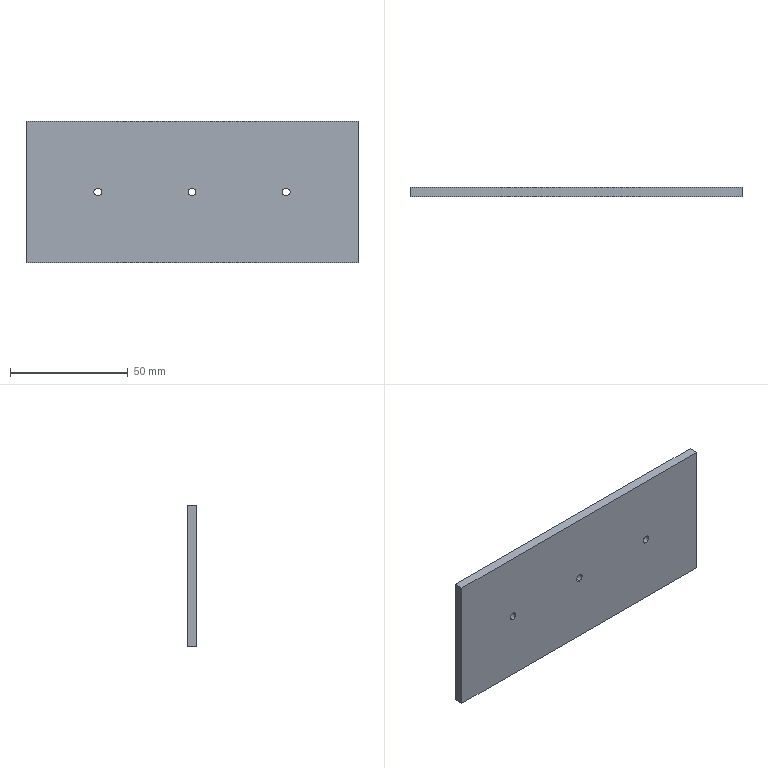Part | SolidWorks | features Extrusion 1, HoleWzd 1 | 1 solid | 12 faces | box 141 x 4 x 60 mm | volume 33737 mm3 | cylinder 6 | plane 6 | commonest cylinder face diameters 3.3 x6
STEP:
#1=CARTESIAN_POINT('',(-40.,0.,-1.65));
#2=VERTEX_POINT('',#1);
#3=CARTESIAN_POINT('',(-40.,0.,1.65));
#4=VERTEX_POINT('',#3);
#5=CARTESIAN_POINT('',(-40.,0.,0.));
#6=DIRECTION('',(0.,1.,0.));
#7=DIRECTION('',(0.,0.,1.));
#8=AXIS2_PLACEMENT_3D('',#5,#6,#7);
#9=CIRCLE('',#8,1.65);
#10=EDGE_CURVE('',#2,#4,#9,.T.);
#11=ORIENTED_EDGE('',*,*,#10,.F.);
#12=CARTESIAN_POINT('',(-40.,4.,-1.65));
#13=VERTEX_POINT('',#12);
#14=CARTESIAN_POINT('',(-40.,4.,-1.65));
#15=DIRECTION('',(0.,1.,0.));
#16=VECTOR('',#15,1000.);
#17=LINE('',#14,#16);
#18=EDGE_CURVE('',#2,#13,#17,.T.);
#19=ORIENTED_EDGE('',*,*,#18,.T.);
#20=CARTESIAN_POINT('',(-40.,4.,1.65));
#21=VERTEX_POINT('',#20);
#22=CARTESIAN_POINT('',(-40.,4.,0.));
#23=DIRECTION('',(0.,1.,0.));
#24=DIRECTION('',(0.,0.,1.));
#25=AXIS2_PLACEMENT_3D('',#22,#23,#24);
#26=CIRCLE('',#25,1.65);
#27=EDGE_CURVE('',#13,#21,#26,.T.);
#28=ORIENTED_EDGE('',*,*,#27,.T.);
#29=CARTESIAN_POINT('',(-40.,4.,1.65));
#30=DIRECTION('',(0.,1.,0.));
#31=VECTOR('',#30,1000.);
#32=LINE('',#29,#31);
#33=EDGE_CURVE('',#4,#21,#32,.T.);
#34=ORIENTED_EDGE('',*,*,#33,.F.);
#35=EDGE_LOOP('',(#11,#19,#28,#34));
#36=FACE_OUTER_BOUND('',#35,.T.);
#37=CARTESIAN_POINT('',(-40.,4.,0.));
#38=DIRECTION('',(0.,1.,0.));
#39=DIRECTION('',(0.,0.,1.));
#40=AXIS2_PLACEMENT_3D('',#37,#38,#39);
#41=CYLINDRICAL_SURFACE('',#40,1.65);
#42=ADVANCED_FACE('',(#36),#41,.F.);
#43=CARTESIAN_POINT('',(0.,0.,-1.65));
#44=VERTEX_POINT('',#43);
#45=CARTESIAN_POINT('',(0.,0.,1.65));
#46=VERTEX_POINT('',#45);
#47=CARTESIAN_POINT('',(0.,0.,0.));
#48=DIRECTION('',(0.,1.,0.));
#49=DIRECTION('',(0.,0.,1.));
#50=AXIS2_PLACEMENT_3D('',#47,#48,#49);
#51=CIRCLE('',#50,1.65);
#52=EDGE_CURVE('',#44,#46,#51,.T.);
#53=ORIENTED_EDGE('',*,*,#52,.F.);
#54=CARTESIAN_POINT('',(0.,4.,-1.65));
#55=VERTEX_POINT('',#54);
#56=CARTESIAN_POINT('',(0.,4.,-1.65));
#57=DIRECTION('',(0.,1.,0.));
#58=VECTOR('',#57,1000.);
#59=LINE('',#56,#58);
#60=EDGE_CURVE('',#44,#55,#59,.T.);
#61=ORIENTED_EDGE('',*,*,#60,.T.);
#62=CARTESIAN_POINT('',(0.,4.,1.65));
#63=VERTEX_POINT('',#62);
#64=CARTESIAN_POINT('',(0.,4.,0.));
#65=DIRECTION('',(0.,1.,0.));
#66=DIRECTION('',(0.,0.,1.));
#67=AXIS2_PLACEMENT_3D('',#64,#65,#66);
#68=CIRCLE('',#67,1.65);
#69=EDGE_CURVE('',#55,#63,#68,.T.);
#70=ORIENTED_EDGE('',*,*,#69,.T.);
#71=CARTESIAN_POINT('',(0.,4.,1.65));
#72=DIRECTION('',(0.,1.,0.));
#73=VECTOR('',#72,1000.);
#74=LINE('',#71,#73);
#75=EDGE_CURVE('',#46,#63,#74,.T.);
#76=ORIENTED_EDGE('',*,*,#75,.F.);
#77=EDGE_LOOP('',(#53,#61,#70,#76));
#78=FACE_OUTER_BOUND('',#77,.T.);
#79=CARTESIAN_POINT('',(0.,4.,0.));
#80=DIRECTION('',(0.,1.,0.));
#81=DIRECTION('',(0.,0.,1.));
#82=AXIS2_PLACEMENT_3D('',#79,#80,#81);
#83=CYLINDRICAL_SURFACE('',#82,1.65);
#84=ADVANCED_FACE('',(#78),#83,.F.);
#85=CARTESIAN_POINT('',(40.,0.,-1.65));
#86=VERTEX_POINT('',#85);
#87=CARTESIAN_POINT('',(40.,0.,1.65));
#88=VERTEX_POINT('',#87);
#89=CARTESIAN_POINT('',(40.,0.,0.));
#90=DIRECTION('',(0.,1.,0.));
#91=DIRECTION('',(0.,0.,1.));
#92=AXIS2_PLACEMENT_3D('',#89,#90,#91);
#93=CIRCLE('',#92,1.65);
#94=EDGE_CURVE('',#86,#88,#93,.T.);
#95=ORIENTED_EDGE('',*,*,#94,.F.);
#96=CARTESIAN_POINT('',(40.,4.,-1.65));
#97=VERTEX_POINT('',#96);
#98=CARTESIAN_POINT('',(40.,4.,-1.65));
#99=DIRECTION('',(0.,1.,0.));
#100=VECTOR('',#99,1000.);
#101=LINE('',#98,#100);
#102=EDGE_CURVE('',#86,#97,#101,.T.);
#103=ORIENTED_EDGE('',*,*,#102,.T.);
#104=CARTESIAN_POINT('',(40.,4.,1.65));
#105=VERTEX_POINT('',#104);
#106=CARTESIAN_POINT('',(40.,4.,0.));
#107=DIRECTION('',(0.,1.,0.));
#108=DIRECTION('',(0.,0.,1.));
#109=AXIS2_PLACEMENT_3D('',#106,#107,#108);
#110=CIRCLE('',#109,1.65);
#111=EDGE_CURVE('',#97,#105,#110,.T.);
#112=ORIENTED_EDGE('',*,*,#111,.T.);
#113=CARTESIAN_POINT('',(40.,4.,1.65));
#114=DIRECTION('',(0.,1.,0.));
#115=VECTOR('',#114,1000.);
#116=LINE('',#113,#115);
#117=EDGE_CURVE('',#88,#105,#116,.T.);
#118=ORIENTED_EDGE('',*,*,#117,.F.);
#119=EDGE_LOOP('',(#95,#103,#112,#118));
#120=FACE_OUTER_BOUND('',#119,.T.);
#121=CARTESIAN_POINT('',(40.,4.,0.));
#122=DIRECTION('',(0.,1.,0.));
#123=DIRECTION('',(0.,0.,1.));
#124=AXIS2_PLACEMENT_3D('',#121,#122,#123);
#125=CYLINDRICAL_SURFACE('',#124,1.65);
#126=ADVANCED_FACE('',(#120),#125,.F.);
#127=CARTESIAN_POINT('',(70.5,0.,30.));
#128=VERTEX_POINT('',#127);
#129=CARTESIAN_POINT('',(70.5,0.,-30.));
#130=VERTEX_POINT('',#129);
#131=CARTESIAN_POINT('',(70.5,0.,-30.));
#132=DIRECTION('',(0.,0.,-1.));
#133=VECTOR('',#132,1000.);
#134=LINE('',#131,#133);
#135=EDGE_CURVE('',#128,#130,#134,.T.);
#136=ORIENTED_EDGE('',*,*,#135,.T.);
#137=CARTESIAN_POINT('',(70.5,4.,-30.));
#138=VERTEX_POINT('',#137);
#139=CARTESIAN_POINT('',(70.5,4.,-30.));
#140=DIRECTION('',(0.,-1.,0.));
#141=VECTOR('',#140,1000.);
#142=LINE('',#139,#141);
#143=EDGE_CURVE('',#138,#130,#142,.T.);
#144=ORIENTED_EDGE('',*,*,#143,.F.);
#145=CARTESIAN_POINT('',(70.5,4.,30.));
#146=VERTEX_POINT('',#145);
#147=CARTESIAN_POINT('',(70.5,4.,-30.));
#148=DIRECTION('',(0.,0.,-1.));
#149=VECTOR('',#148,1000.);
#150=LINE('',#147,#149);
#151=EDGE_CURVE('',#146,#138,#150,.T.);
#152=ORIENTED_EDGE('',*,*,#151,.F.);
#153=CARTESIAN_POINT('',(70.5,4.,30.));
#154=DIRECTION('',(0.,-1.,0.));
#155=VECTOR('',#154,1000.);
#156=LINE('',#153,#155);
#157=EDGE_CURVE('',#146,#128,#156,.T.);
#158=ORIENTED_EDGE('',*,*,#157,.T.);
#159=EDGE_LOOP('',(#136,#144,#152,#158));
#160=FACE_OUTER_BOUND('',#159,.T.);
#161=CARTESIAN_POINT('',(70.5,4.,-30.));
#162=DIRECTION('',(-1.,0.,0.));
#163=DIRECTION('',(0.,0.,1.));
#164=AXIS2_PLACEMENT_3D('',#161,#162,#163);
#165=PLANE('',#164);
#166=ADVANCED_FACE('',(#160),#165,.F.);
#167=CARTESIAN_POINT('',(-70.5,0.,-30.));
#168=VERTEX_POINT('',#167);
#169=CARTESIAN_POINT('',(-70.5,0.,-30.));
#170=DIRECTION('',(-1.,0.,0.));
#171=VECTOR('',#170,1000.);
#172=LINE('',#169,#171);
#173=EDGE_CURVE('',#130,#168,#172,.T.);
#174=ORIENTED_EDGE('',*,*,#173,.T.);
#175=CARTESIAN_POINT('',(-70.5,4.,-30.));
#176=VERTEX_POINT('',#175);
#177=CARTESIAN_POINT('',(-70.5,4.,-30.));
#178=DIRECTION('',(0.,-1.,0.));
#179=VECTOR('',#178,1000.);
#180=LINE('',#177,#179);
#181=EDGE_CURVE('',#176,#168,#180,.T.);
#182=ORIENTED_EDGE('',*,*,#181,.F.);
#183=CARTESIAN_POINT('',(-70.5,4.,-30.));
#184=DIRECTION('',(-1.,0.,0.));
#185=VECTOR('',#184,1000.);
#186=LINE('',#183,#185);
#187=EDGE_CURVE('',#138,#176,#186,.T.);
#188=ORIENTED_EDGE('',*,*,#187,.F.);
#189=ORIENTED_EDGE('',*,*,#143,.T.);
#190=EDGE_LOOP('',(#174,#182,#188,#189));
#191=FACE_OUTER_BOUND('',#190,.T.);
#192=CARTESIAN_POINT('',(-70.5,4.,-30.));
#193=DIRECTION('',(0.,0.,1.));
#194=DIRECTION('',(1.,0.,0.));
#195=AXIS2_PLACEMENT_3D('',#192,#193,#194);
#196=PLANE('',#195);
#197=ADVANCED_FACE('',(#191),#196,.F.);
#198=CARTESIAN_POINT('',(-70.5,0.,30.));
#199=VERTEX_POINT('',#198);
#200=CARTESIAN_POINT('',(-70.5,0.,-30.));
#201=DIRECTION('',(0.,0.,1.));
#202=VECTOR('',#201,1000.);
#203=LINE('',#200,#202);
#204=EDGE_CURVE('',#168,#199,#203,.T.);
#205=ORIENTED_EDGE('',*,*,#204,.T.);
#206=CARTESIAN_POINT('',(-70.5,4.,30.));
#207=VERTEX_POINT('',#206);
#208=CARTESIAN_POINT('',(-70.5,4.,30.));
#209=DIRECTION('',(0.,-1.,0.));
#210=VECTOR('',#209,1000.);
#211=LINE('',#208,#210);
#212=EDGE_CURVE('',#207,#199,#211,.T.);
#213=ORIENTED_EDGE('',*,*,#212,.F.);
#214=CARTESIAN_POINT('',(-70.5,4.,-30.));
#215=DIRECTION('',(0.,0.,1.));
#216=VECTOR('',#215,1000.);
#217=LINE('',#214,#216);
#218=EDGE_CURVE('',#176,#207,#217,.T.);
#219=ORIENTED_EDGE('',*,*,#218,.F.);
#220=ORIENTED_EDGE('',*,*,#181,.T.);
#221=EDGE_LOOP('',(#205,#213,#219,#220));
#222=FACE_OUTER_BOUND('',#221,.T.);
#223=CARTESIAN_POINT('',(-70.5,4.,-30.));
#224=DIRECTION('',(1.,0.,0.));
#225=DIRECTION('',(0.,0.,-1.));
#226=AXIS2_PLACEMENT_3D('',#223,#224,#225);
#227=PLANE('',#226);
#228=ADVANCED_FACE('',(#222),#227,.F.);
#229=CARTESIAN_POINT('',(-70.5,0.,30.));
#230=DIRECTION('',(1.,0.,0.));
#231=VECTOR('',#230,1000.);
#232=LINE('',#229,#231);
#233=EDGE_CURVE('',#199,#128,#232,.T.);
#234=ORIENTED_EDGE('',*,*,#233,.T.);
#235=ORIENTED_EDGE('',*,*,#157,.F.);
#236=CARTESIAN_POINT('',(-70.5,4.,30.));
#237=DIRECTION('',(1.,0.,0.));
#238=VECTOR('',#237,1000.);
#239=LINE('',#236,#238);
#240=EDGE_CURVE('',#207,#146,#239,.T.);
#241=ORIENTED_EDGE('',*,*,#240,.F.);
#242=ORIENTED_EDGE('',*,*,#212,.T.);
#243=EDGE_LOOP('',(#234,#235,#241,#242));
#244=FACE_OUTER_BOUND('',#243,.T.);
#245=CARTESIAN_POINT('',(-70.5,4.,30.));
#246=DIRECTION('',(0.,0.,-1.));
#247=DIRECTION('',(-1.,0.,0.));
#248=AXIS2_PLACEMENT_3D('',#245,#246,#247);
#249=PLANE('',#248);
#250=ADVANCED_FACE('',(#244),#249,.F.);
#251=CARTESIAN_POINT('',(-40.,4.,0.));
#252=DIRECTION('',(0.,1.,0.));
#253=DIRECTION('',(0.,0.,1.));
#254=AXIS2_PLACEMENT_3D('',#251,#252,#253);
#255=CIRCLE('',#254,1.65);
#256=EDGE_CURVE('',#21,#13,#255,.T.);
#257=ORIENTED_EDGE('',*,*,#256,.F.);
#258=ORIENTED_EDGE('',*,*,#27,.F.);
#259=EDGE_LOOP('',(#257,#258));
#260=FACE_BOUND('',#259,.T.);
#261=CARTESIAN_POINT('',(0.,4.,0.));
#262=DIRECTION('',(0.,1.,0.));
#263=DIRECTION('',(0.,0.,1.));
#264=AXIS2_PLACEMENT_3D('',#261,#262,#263);
#265=CIRCLE('',#264,1.65);
#266=EDGE_CURVE('',#63,#55,#265,.T.);
#267=ORIENTED_EDGE('',*,*,#266,.F.);
#268=ORIENTED_EDGE('',*,*,#69,.F.);
#269=EDGE_LOOP('',(#267,#268));
#270=FACE_BOUND('',#269,.T.);
#271=CARTESIAN_POINT('',(40.,4.,0.));
#272=DIRECTION('',(0.,1.,0.));
#273=DIRECTION('',(0.,0.,1.));
#274=AXIS2_PLACEMENT_3D('',#271,#272,#273);
#275=CIRCLE('',#274,1.65);
#276=EDGE_CURVE('',#105,#97,#275,.T.);
#277=ORIENTED_EDGE('',*,*,#276,.F.);
#278=ORIENTED_EDGE('',*,*,#111,.F.);
#279=EDGE_LOOP('',(#277,#278));
#280=FACE_BOUND('',#279,.T.);
#281=ORIENTED_EDGE('',*,*,#151,.T.);
#282=ORIENTED_EDGE('',*,*,#187,.T.);
#283=ORIENTED_EDGE('',*,*,#218,.T.);
#284=ORIENTED_EDGE('',*,*,#240,.T.);
#285=EDGE_LOOP('',(#281,#282,#283,#284));
#286=FACE_OUTER_BOUND('',#285,.T.);
#287=CARTESIAN_POINT('',(0.,4.,0.));
#288=DIRECTION('',(0.,1.,0.));
#289=DIRECTION('',(0.,0.,1.));
#290=AXIS2_PLACEMENT_3D('',#287,#288,#289);
#291=PLANE('',#290);
#292=ADVANCED_FACE('',(#260,#270,#280,#286),#291,.T.);
#293=CARTESIAN_POINT('',(-40.,0.,0.));
#294=DIRECTION('',(0.,1.,0.));
#295=DIRECTION('',(0.,0.,1.));
#296=AXIS2_PLACEMENT_3D('',#293,#294,#295);
#297=CIRCLE('',#296,1.65);
#298=EDGE_CURVE('',#4,#2,#297,.T.);
#299=ORIENTED_EDGE('',*,*,#298,.T.);
#300=ORIENTED_EDGE('',*,*,#10,.T.);
#301=EDGE_LOOP('',(#299,#300));
#302=FACE_BOUND('',#301,.T.);
#303=CARTESIAN_POINT('',(0.,0.,0.));
#304=DIRECTION('',(0.,1.,0.));
#305=DIRECTION('',(0.,0.,1.));
#306=AXIS2_PLACEMENT_3D('',#303,#304,#305);
#307=CIRCLE('',#306,1.65);
#308=EDGE_CURVE('',#46,#44,#307,.T.);
#309=ORIENTED_EDGE('',*,*,#308,.T.);
#310=ORIENTED_EDGE('',*,*,#52,.T.);
#311=EDGE_LOOP('',(#309,#310));
#312=FACE_BOUND('',#311,.T.);
#313=CARTESIAN_POINT('',(40.,0.,0.));
#314=DIRECTION('',(0.,1.,0.));
#315=DIRECTION('',(0.,0.,1.));
#316=AXIS2_PLACEMENT_3D('',#313,#314,#315);
#317=CIRCLE('',#316,1.65);
#318=EDGE_CURVE('',#88,#86,#317,.T.);
#319=ORIENTED_EDGE('',*,*,#318,.T.);
#320=ORIENTED_EDGE('',*,*,#94,.T.);
#321=EDGE_LOOP('',(#319,#320));
#322=FACE_BOUND('',#321,.T.);
#323=ORIENTED_EDGE('',*,*,#135,.F.);
#324=ORIENTED_EDGE('',*,*,#233,.F.);
#325=ORIENTED_EDGE('',*,*,#204,.F.);
#326=ORIENTED_EDGE('',*,*,#173,.F.);
#327=EDGE_LOOP('',(#323,#324,#325,#326));
#328=FACE_OUTER_BOUND('',#327,.T.);
#329=CARTESIAN_POINT('',(0.,0.,0.));
#330=DIRECTION('',(0.,1.,0.));
#331=DIRECTION('',(0.,0.,1.));
#332=AXIS2_PLACEMENT_3D('',#329,#330,#331);
#333=PLANE('',#332);
#334=ADVANCED_FACE('',(#302,#312,#322,#328),#333,.F.);
#335=ORIENTED_EDGE('',*,*,#102,.F.);
#336=ORIENTED_EDGE('',*,*,#318,.F.);
#337=ORIENTED_EDGE('',*,*,#117,.T.);
#338=ORIENTED_EDGE('',*,*,#276,.T.);
#339=EDGE_LOOP('',(#335,#336,#337,#338));
#340=FACE_OUTER_BOUND('',#339,.T.);
#341=CARTESIAN_POINT('',(40.,4.,0.));
#342=DIRECTION('',(0.,1.,0.));
#343=DIRECTION('',(0.,0.,1.));
#344=AXIS2_PLACEMENT_3D('',#341,#342,#343);
#345=CYLINDRICAL_SURFACE('',#344,1.65);
#346=ADVANCED_FACE('',(#340),#345,.F.);
#347=ORIENTED_EDGE('',*,*,#60,.F.);
#348=ORIENTED_EDGE('',*,*,#308,.F.);
#349=ORIENTED_EDGE('',*,*,#75,.T.);
#350=ORIENTED_EDGE('',*,*,#266,.T.);
#351=EDGE_LOOP('',(#347,#348,#349,#350));
#352=FACE_OUTER_BOUND('',#351,.T.);
#353=CARTESIAN_POINT('',(0.,4.,0.));
#354=DIRECTION('',(0.,1.,0.));
#355=DIRECTION('',(0.,0.,1.));
#356=AXIS2_PLACEMENT_3D('',#353,#354,#355);
#357=CYLINDRICAL_SURFACE('',#356,1.65);
#358=ADVANCED_FACE('',(#352),#357,.F.);
#359=ORIENTED_EDGE('',*,*,#18,.F.);
#360=ORIENTED_EDGE('',*,*,#298,.F.);
#361=ORIENTED_EDGE('',*,*,#33,.T.);
#362=ORIENTED_EDGE('',*,*,#256,.T.);
#363=EDGE_LOOP('',(#359,#360,#361,#362));
#364=FACE_OUTER_BOUND('',#363,.T.);
#365=CARTESIAN_POINT('',(-40.,4.,0.));
#366=DIRECTION('',(0.,1.,0.));
#367=DIRECTION('',(0.,0.,1.));
#368=AXIS2_PLACEMENT_3D('',#365,#366,#367);
#369=CYLINDRICAL_SURFACE('',#368,1.65);
#370=ADVANCED_FACE('',(#364),#369,.F.);
#371=CLOSED_SHELL('',(#42,#84,#126,#166,#197,#228,#250,#292,#334,#346,#358,#370));
#372=MANIFOLD_SOLID_BREP('',#371);
#373=CARTESIAN_POINT('',(0.,0.,0.));
#374=DIRECTION('',(0.,0.,1.));
#375=DIRECTION('',(1.,0.,0.));
#376=AXIS2_PLACEMENT_3D('',#373,#374,#375);
#377=(LENGTH_UNIT()NAMED_UNIT(*)SI_UNIT(.MILLI.,.METRE.));
#378=UNCERTAINTY_MEASURE_WITH_UNIT(LENGTH_MEASURE(0.00001),#377,'','');
#379=(NAMED_UNIT(*)PLANE_ANGLE_UNIT()SI_UNIT($,.RADIAN.));
#380=(NAMED_UNIT(*)SI_UNIT($,.STERADIAN.)SOLID_ANGLE_UNIT());
#381=(GEOMETRIC_REPRESENTATION_CONTEXT(3)GLOBAL_UNCERTAINTY_ASSIGNED_CONTEXT((#378))GLOBAL_UNIT_ASSIGNED_CONTEXT((#377,#379,#380))REPRESENTATION_CONTEXT('',''));
#382=ADVANCED_BREP_SHAPE_REPRESENTATION('',(#372,#376),#381);